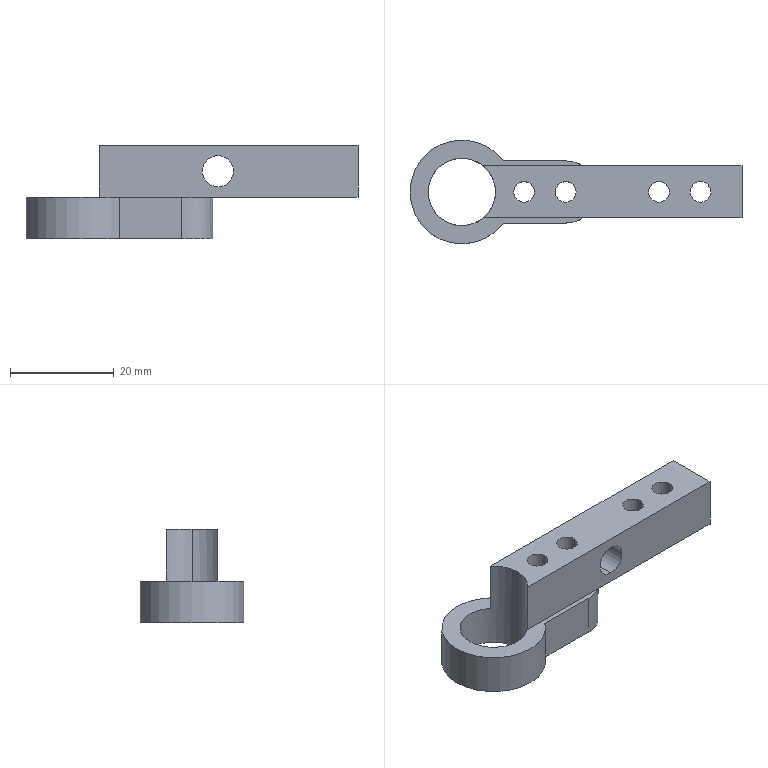Part | SolidWorks | features ICE 6, Extrusion 1 | 1 solid | 24 faces | box 64 x 20 x 18 mm | volume 6760 mm3 | cylinder 15 | plane 9 | commonest cylinder face diameters 4 x8 6 x2 12 x2 13 x2 20 x1
STEP:
#1=CARTESIAN_POINT('',(2.5,5.,10.));
#2=VERTEX_POINT('',#1);
#3=CARTESIAN_POINT('',(0.1533,0.,10.));
#4=VERTEX_POINT('',#3);
#5=CARTESIAN_POINT('',(-4.,5.,10.));
#6=DIRECTION('',(0.,0.,-1.));
#7=DIRECTION('',(-1.,0.,0.));
#8=AXIS2_PLACEMENT_3D('',#5,#6,#7);
#9=CIRCLE('',#8,6.5);
#10=EDGE_CURVE('',#2,#4,#9,.T.);
#11=ORIENTED_EDGE('',*,*,#10,.F.);
#12=CARTESIAN_POINT('',(2.5,5.,-8.));
#13=VERTEX_POINT('',#12);
#14=CARTESIAN_POINT('',(2.5,5.,10.));
#15=DIRECTION('',(0.,0.,-1.));
#16=VECTOR('',#15,1000.);
#17=LINE('',#14,#16);
#18=EDGE_CURVE('',#2,#13,#17,.T.);
#19=ORIENTED_EDGE('',*,*,#18,.T.);
#20=CARTESIAN_POINT('',(-10.5,5.,-8.));
#21=VERTEX_POINT('',#20);
#22=CARTESIAN_POINT('',(-4.,5.,-8.));
#23=DIRECTION('',(0.,0.,1.));
#24=DIRECTION('',(1.,0.,0.));
#25=AXIS2_PLACEMENT_3D('',#22,#23,#24);
#26=CIRCLE('',#25,6.5);
#27=EDGE_CURVE('',#21,#13,#26,.T.);
#28=ORIENTED_EDGE('',*,*,#27,.F.);
#29=CARTESIAN_POINT('',(-10.5,5.,0.));
#30=VERTEX_POINT('',#29);
#31=CARTESIAN_POINT('',(-10.5,5.,10.));
#32=DIRECTION('',(0.,0.,-1.));
#33=VECTOR('',#32,1000.);
#34=LINE('',#31,#33);
#35=EDGE_CURVE('',#30,#21,#34,.T.);
#36=ORIENTED_EDGE('',*,*,#35,.F.);
#37=CARTESIAN_POINT('',(0.1533,0.,0.));
#38=VERTEX_POINT('',#37);
#39=CARTESIAN_POINT('',(-4.,5.,0.));
#40=DIRECTION('',(0.,0.,-1.));
#41=DIRECTION('',(-1.,0.,0.));
#42=AXIS2_PLACEMENT_3D('',#39,#40,#41);
#43=CIRCLE('',#42,6.5);
#44=EDGE_CURVE('',#38,#30,#43,.T.);
#45=ORIENTED_EDGE('',*,*,#44,.F.);
#46=CARTESIAN_POINT('',(0.1533,0.,10.));
#47=DIRECTION('',(0.,0.,-1.));
#48=VECTOR('',#47,1000.);
#49=LINE('',#46,#48);
#50=EDGE_CURVE('',#4,#38,#49,.T.);
#51=ORIENTED_EDGE('',*,*,#50,.F.);
#52=EDGE_LOOP('',(#11,#19,#28,#36,#45,#51));
#53=FACE_OUTER_BOUND('',#52,.T.);
#54=CARTESIAN_POINT('',(-4.,5.,10.));
#55=DIRECTION('',(0.,0.,-1.));
#56=DIRECTION('',(-1.,0.,0.));
#57=AXIS2_PLACEMENT_3D('',#54,#55,#56);
#58=CYLINDRICAL_SURFACE('',#57,6.5);
#59=ADVANCED_FACE('',(#53),#58,.F.);
#60=CARTESIAN_POINT('',(16.,-1.,-8.));
#61=VERTEX_POINT('',#60);
#62=CARTESIAN_POINT('',(22.,5.,-8.));
#63=VERTEX_POINT('',#62);
#64=CARTESIAN_POINT('',(16.,5.,-8.));
#65=DIRECTION('',(0.,0.,1.));
#66=DIRECTION('',(1.,0.,0.));
#67=AXIS2_PLACEMENT_3D('',#64,#65,#66);
#68=CIRCLE('',#67,6.);
#69=EDGE_CURVE('',#61,#63,#68,.T.);
#70=ORIENTED_EDGE('',*,*,#69,.T.);
#71=CARTESIAN_POINT('',(22.,5.,0.));
#72=VERTEX_POINT('',#71);
#73=CARTESIAN_POINT('',(22.,5.,-30.));
#74=DIRECTION('',(0.,0.,1.));
#75=VECTOR('',#74,1000.);
#76=LINE('',#73,#75);
#77=EDGE_CURVE('',#63,#72,#76,.T.);
#78=ORIENTED_EDGE('',*,*,#77,.T.);
#79=CARTESIAN_POINT('',(19.317,0.,0.));
#80=VERTEX_POINT('',#79);
#81=CARTESIAN_POINT('',(16.,5.,0.));
#82=DIRECTION('',(0.,0.,-1.));
#83=DIRECTION('',(-1.,0.,0.));
#84=AXIS2_PLACEMENT_3D('',#81,#82,#83);
#85=CIRCLE('',#84,6.);
#86=EDGE_CURVE('',#72,#80,#85,.T.);
#87=ORIENTED_EDGE('',*,*,#86,.T.);
#88=CARTESIAN_POINT('',(16.,-1.,0.));
#89=VERTEX_POINT('',#88);
#90=CARTESIAN_POINT('',(16.,5.,0.));
#91=DIRECTION('',(0.,0.,-1.));
#92=DIRECTION('',(-1.,0.,0.));
#93=AXIS2_PLACEMENT_3D('',#90,#91,#92);
#94=CIRCLE('',#93,6.);
#95=EDGE_CURVE('',#80,#89,#94,.T.);
#96=ORIENTED_EDGE('',*,*,#95,.T.);
#97=CARTESIAN_POINT('',(16.,-1.,-30.));
#98=DIRECTION('',(0.,0.,1.));
#99=VECTOR('',#98,1000.);
#100=LINE('',#97,#99);
#101=EDGE_CURVE('',#61,#89,#100,.T.);
#102=ORIENTED_EDGE('',*,*,#101,.F.);
#103=EDGE_LOOP('',(#70,#78,#87,#96,#102));
#104=FACE_OUTER_BOUND('',#103,.T.);
#105=CARTESIAN_POINT('',(16.,5.,-30.));
#106=DIRECTION('',(0.,0.,1.));
#107=DIRECTION('',(1.,0.,0.));
#108=AXIS2_PLACEMENT_3D('',#105,#106,#107);
#109=CYLINDRICAL_SURFACE('',#108,6.);
#110=ADVANCED_FACE('',(#104),#109,.T.);
#111=CARTESIAN_POINT('',(6.,5.,-8.));
#112=VERTEX_POINT('',#111);
#113=CARTESIAN_POINT('',(10.,5.,-8.));
#114=VERTEX_POINT('',#113);
#115=CARTESIAN_POINT('',(8.,5.,-8.));
#116=DIRECTION('',(0.,0.,1.));
#117=DIRECTION('',(1.,0.,0.));
#118=AXIS2_PLACEMENT_3D('',#115,#116,#117);
#119=CIRCLE('',#118,2.);
#120=EDGE_CURVE('',#112,#114,#119,.T.);
#121=ORIENTED_EDGE('',*,*,#120,.F.);
#122=CARTESIAN_POINT('',(6.,5.,10.));
#123=VERTEX_POINT('',#122);
#124=CARTESIAN_POINT('',(6.,5.,0.));
#125=DIRECTION('',(0.,0.,1.));
#126=VECTOR('',#125,1000.);
#127=LINE('',#124,#126);
#128=EDGE_CURVE('',#112,#123,#127,.T.);
#129=ORIENTED_EDGE('',*,*,#128,.T.);
#130=CARTESIAN_POINT('',(10.,5.,10.));
#131=VERTEX_POINT('',#130);
#132=CARTESIAN_POINT('',(8.,5.,10.));
#133=DIRECTION('',(0.,0.,1.));
#134=DIRECTION('',(1.,0.,0.));
#135=AXIS2_PLACEMENT_3D('',#132,#133,#134);
#136=CIRCLE('',#135,2.);
#137=EDGE_CURVE('',#123,#131,#136,.T.);
#138=ORIENTED_EDGE('',*,*,#137,.T.);
#139=CARTESIAN_POINT('',(10.,5.,0.));
#140=DIRECTION('',(0.,0.,1.));
#141=VECTOR('',#140,1000.);
#142=LINE('',#139,#141);
#143=EDGE_CURVE('',#114,#131,#142,.T.);
#144=ORIENTED_EDGE('',*,*,#143,.F.);
#145=EDGE_LOOP('',(#121,#129,#138,#144));
#146=FACE_OUTER_BOUND('',#145,.T.);
#147=CARTESIAN_POINT('',(8.,5.,0.));
#148=DIRECTION('',(0.,0.,1.));
#149=DIRECTION('',(1.,0.,0.));
#150=AXIS2_PLACEMENT_3D('',#147,#148,#149);
#151=CYLINDRICAL_SURFACE('',#150,2.);
#152=ADVANCED_FACE('',(#146),#151,.F.);
#153=CARTESIAN_POINT('',(32.,5.,0.));
#154=VERTEX_POINT('',#153);
#155=CARTESIAN_POINT('',(36.,5.,0.));
#156=VERTEX_POINT('',#155);
#157=CARTESIAN_POINT('',(34.,5.,0.));
#158=DIRECTION('',(0.,0.,1.));
#159=DIRECTION('',(-1.,0.,0.));
#160=AXIS2_PLACEMENT_3D('',#157,#158,#159);
#161=CIRCLE('',#160,2.);
#162=EDGE_CURVE('',#154,#156,#161,.T.);
#163=ORIENTED_EDGE('',*,*,#162,.F.);
#164=CARTESIAN_POINT('',(32.,5.,10.));
#165=VERTEX_POINT('',#164);
#166=CARTESIAN_POINT('',(32.,5.,0.));
#167=DIRECTION('',(0.,0.,1.));
#168=VECTOR('',#167,1000.);
#169=LINE('',#166,#168);
#170=EDGE_CURVE('',#154,#165,#169,.T.);
#171=ORIENTED_EDGE('',*,*,#170,.T.);
#172=CARTESIAN_POINT('',(36.,5.,10.));
#173=VERTEX_POINT('',#172);
#174=CARTESIAN_POINT('',(34.,5.,10.));
#175=DIRECTION('',(0.,0.,1.));
#176=DIRECTION('',(-1.,0.,0.));
#177=AXIS2_PLACEMENT_3D('',#174,#175,#176);
#178=CIRCLE('',#177,2.);
#179=EDGE_CURVE('',#165,#173,#178,.T.);
#180=ORIENTED_EDGE('',*,*,#179,.T.);
#181=CARTESIAN_POINT('',(36.,5.,0.));
#182=DIRECTION('',(0.,0.,1.));
#183=VECTOR('',#182,1000.);
#184=LINE('',#181,#183);
#185=EDGE_CURVE('',#156,#173,#184,.T.);
#186=ORIENTED_EDGE('',*,*,#185,.F.);
#187=EDGE_LOOP('',(#163,#171,#180,#186));
#188=FACE_OUTER_BOUND('',#187,.T.);
#189=CARTESIAN_POINT('',(34.,5.,0.));
#190=DIRECTION('',(0.,0.,1.));
#191=DIRECTION('',(1.,0.,0.));
#192=AXIS2_PLACEMENT_3D('',#189,#190,#191);
#193=CYLINDRICAL_SURFACE('',#192,2.);
#194=ADVANCED_FACE('',(#188),#193,.F.);
#195=CARTESIAN_POINT('',(40.,5.,0.));
#196=VERTEX_POINT('',#195);
#197=CARTESIAN_POINT('',(44.,5.,0.));
#198=VERTEX_POINT('',#197);
#199=CARTESIAN_POINT('',(42.,5.,0.));
#200=DIRECTION('',(0.,0.,1.));
#201=DIRECTION('',(-1.,0.,0.));
#202=AXIS2_PLACEMENT_3D('',#199,#200,#201);
#203=CIRCLE('',#202,2.);
#204=EDGE_CURVE('',#196,#198,#203,.T.);
#205=ORIENTED_EDGE('',*,*,#204,.F.);
#206=CARTESIAN_POINT('',(40.,5.,10.));
#207=VERTEX_POINT('',#206);
#208=CARTESIAN_POINT('',(40.,5.,0.));
#209=DIRECTION('',(0.,0.,1.));
#210=VECTOR('',#209,1000.);
#211=LINE('',#208,#210);
#212=EDGE_CURVE('',#196,#207,#211,.T.);
#213=ORIENTED_EDGE('',*,*,#212,.T.);
#214=CARTESIAN_POINT('',(44.,5.,10.));
#215=VERTEX_POINT('',#214);
#216=CARTESIAN_POINT('',(42.,5.,10.));
#217=DIRECTION('',(0.,0.,1.));
#218=DIRECTION('',(-1.,0.,0.));
#219=AXIS2_PLACEMENT_3D('',#216,#217,#218);
#220=CIRCLE('',#219,2.);
#221=EDGE_CURVE('',#207,#215,#220,.T.);
#222=ORIENTED_EDGE('',*,*,#221,.T.);
#223=CARTESIAN_POINT('',(44.,5.,0.));
#224=DIRECTION('',(0.,0.,1.));
#225=VECTOR('',#224,1000.);
#226=LINE('',#223,#225);
#227=EDGE_CURVE('',#198,#215,#226,.T.);
#228=ORIENTED_EDGE('',*,*,#227,.F.);
#229=EDGE_LOOP('',(#205,#213,#222,#228));
#230=FACE_OUTER_BOUND('',#229,.T.);
#231=CARTESIAN_POINT('',(42.,5.,0.));
#232=DIRECTION('',(0.,0.,1.));
#233=DIRECTION('',(1.,0.,0.));
#234=AXIS2_PLACEMENT_3D('',#231,#232,#233);
#235=CYLINDRICAL_SURFACE('',#234,2.);
#236=ADVANCED_FACE('',(#230),#235,.F.);
#237=CARTESIAN_POINT('',(14.,5.,-8.));
#238=VERTEX_POINT('',#237);
#239=CARTESIAN_POINT('',(18.,5.,-8.));
#240=VERTEX_POINT('',#239);
#241=CARTESIAN_POINT('',(16.,5.,-8.));
#242=DIRECTION('',(0.,0.,1.));
#243=DIRECTION('',(1.,0.,0.));
#244=AXIS2_PLACEMENT_3D('',#241,#242,#243);
#245=CIRCLE('',#244,2.);
#246=EDGE_CURVE('',#238,#240,#245,.T.);
#247=ORIENTED_EDGE('',*,*,#246,.F.);
#248=CARTESIAN_POINT('',(14.,5.,10.));
#249=VERTEX_POINT('',#248);
#250=CARTESIAN_POINT('',(14.,5.,0.));
#251=DIRECTION('',(0.,0.,1.));
#252=VECTOR('',#251,1000.);
#253=LINE('',#250,#252);
#254=EDGE_CURVE('',#238,#249,#253,.T.);
#255=ORIENTED_EDGE('',*,*,#254,.T.);
#256=CARTESIAN_POINT('',(18.,5.,10.));
#257=VERTEX_POINT('',#256);
#258=CARTESIAN_POINT('',(16.,5.,10.));
#259=DIRECTION('',(0.,0.,1.));
#260=DIRECTION('',(1.,0.,0.));
#261=AXIS2_PLACEMENT_3D('',#258,#259,#260);
#262=CIRCLE('',#261,2.);
#263=EDGE_CURVE('',#249,#257,#262,.T.);
#264=ORIENTED_EDGE('',*,*,#263,.T.);
#265=CARTESIAN_POINT('',(18.,5.,0.));
#266=DIRECTION('',(0.,0.,1.));
#267=VECTOR('',#266,1000.);
#268=LINE('',#265,#267);
#269=EDGE_CURVE('',#240,#257,#268,.T.);
#270=ORIENTED_EDGE('',*,*,#269,.F.);
#271=EDGE_LOOP('',(#247,#255,#264,#270));
#272=FACE_OUTER_BOUND('',#271,.T.);
#273=CARTESIAN_POINT('',(16.,5.,0.));
#274=DIRECTION('',(0.,0.,1.));
#275=DIRECTION('',(1.,0.,0.));
#276=AXIS2_PLACEMENT_3D('',#273,#274,#275);
#277=CYLINDRICAL_SURFACE('',#276,2.);
#278=ADVANCED_FACE('',(#272),#277,.F.);
#279=CARTESIAN_POINT('',(23.,0.,2.));
#280=VERTEX_POINT('',#279);
#281=CARTESIAN_POINT('',(23.,0.,8.));
#282=VERTEX_POINT('',#281);
#283=CARTESIAN_POINT('',(23.,0.,5.));
#284=DIRECTION('',(0.,1.,0.));
#285=DIRECTION('',(0.,0.,1.));
#286=AXIS2_PLACEMENT_3D('',#283,#284,#285);
#287=CIRCLE('',#286,3.);
#288=EDGE_CURVE('',#280,#282,#287,.T.);
#289=ORIENTED_EDGE('',*,*,#288,.F.);
#290=CARTESIAN_POINT('',(23.,10.,2.));
#291=VERTEX_POINT('',#290);
#292=CARTESIAN_POINT('',(23.,0.,2.));
#293=DIRECTION('',(0.,1.,0.));
#294=VECTOR('',#293,1000.);
#295=LINE('',#292,#294);
#296=EDGE_CURVE('',#280,#291,#295,.T.);
#297=ORIENTED_EDGE('',*,*,#296,.T.);
#298=CARTESIAN_POINT('',(23.,10.,8.));
#299=VERTEX_POINT('',#298);
#300=CARTESIAN_POINT('',(23.,10.,5.));
#301=DIRECTION('',(0.,1.,0.));
#302=DIRECTION('',(0.,0.,1.));
#303=AXIS2_PLACEMENT_3D('',#300,#301,#302);
#304=CIRCLE('',#303,3.);
#305=EDGE_CURVE('',#291,#299,#304,.T.);
#306=ORIENTED_EDGE('',*,*,#305,.T.);
#307=CARTESIAN_POINT('',(23.,0.,8.));
#308=DIRECTION('',(0.,1.,0.));
#309=VECTOR('',#308,1000.);
#310=LINE('',#307,#309);
#311=EDGE_CURVE('',#282,#299,#310,.T.);
#312=ORIENTED_EDGE('',*,*,#311,.F.);
#313=EDGE_LOOP('',(#289,#297,#306,#312));
#314=FACE_OUTER_BOUND('',#313,.T.);
#315=CARTESIAN_POINT('',(23.,0.,5.));
#316=DIRECTION('',(0.,1.,0.));
#317=DIRECTION('',(0.,0.,1.));
#318=AXIS2_PLACEMENT_3D('',#315,#316,#317);
#319=CYLINDRICAL_SURFACE('',#318,3.);
#320=ADVANCED_FACE('',(#314),#319,.F.);
#321=CARTESIAN_POINT('',(8.,5.,10.));
#322=DIRECTION('',(0.,0.,1.));
#323=DIRECTION('',(1.,0.,0.));
#324=AXIS2_PLACEMENT_3D('',#321,#322,#323);
#325=CIRCLE('',#324,2.);
#326=EDGE_CURVE('',#131,#123,#325,.T.);
#327=ORIENTED_EDGE('',*,*,#326,.F.);
#328=ORIENTED_EDGE('',*,*,#137,.F.);
#329=EDGE_LOOP('',(#327,#328));
#330=FACE_BOUND('',#329,.T.);
#331=CARTESIAN_POINT('',(34.,5.,10.));
#332=DIRECTION('',(0.,0.,1.));
#333=DIRECTION('',(-1.,0.,0.));
#334=AXIS2_PLACEMENT_3D('',#331,#332,#333);
#335=CIRCLE('',#334,2.);
#336=EDGE_CURVE('',#173,#165,#335,.T.);
#337=ORIENTED_EDGE('',*,*,#336,.F.);
#338=ORIENTED_EDGE('',*,*,#179,.F.);
#339=EDGE_LOOP('',(#337,#338));
#340=FACE_BOUND('',#339,.T.);
#341=CARTESIAN_POINT('',(42.,5.,10.));
#342=DIRECTION('',(0.,0.,1.));
#343=DIRECTION('',(-1.,0.,0.));
#344=AXIS2_PLACEMENT_3D('',#341,#342,#343);
#345=CIRCLE('',#344,2.);
#346=EDGE_CURVE('',#215,#207,#345,.T.);
#347=ORIENTED_EDGE('',*,*,#346,.F.);
#348=ORIENTED_EDGE('',*,*,#221,.F.);
#349=EDGE_LOOP('',(#347,#348));
#350=FACE_BOUND('',#349,.T.);
#351=CARTESIAN_POINT('',(16.,5.,10.));
#352=DIRECTION('',(0.,0.,1.));
#353=DIRECTION('',(1.,0.,0.));
#354=AXIS2_PLACEMENT_3D('',#351,#352,#353);
#355=CIRCLE('',#354,2.);
#356=EDGE_CURVE('',#257,#249,#355,.T.);
#357=ORIENTED_EDGE('',*,*,#356,.F.);
#358=ORIENTED_EDGE('',*,*,#263,.F.);
#359=EDGE_LOOP('',(#357,#358));
#360=FACE_BOUND('',#359,.T.);
#361=CARTESIAN_POINT('',(0.1533,10.,10.));
#362=VERTEX_POINT('',#361);
#363=CARTESIAN_POINT('',(50.,10.,10.));
#364=VERTEX_POINT('',#363);
#365=CARTESIAN_POINT('',(0.,10.,10.));
#366=DIRECTION('',(1.,0.,0.));
#367=VECTOR('',#366,1000.);
#368=LINE('',#365,#367);
#369=EDGE_CURVE('',#362,#364,#368,.T.);
#370=ORIENTED_EDGE('',*,*,#369,.F.);
#371=CARTESIAN_POINT('',(-4.,5.,10.));
#372=DIRECTION('',(0.,0.,-1.));
#373=DIRECTION('',(-1.,0.,0.));
#374=AXIS2_PLACEMENT_3D('',#371,#372,#373);
#375=CIRCLE('',#374,6.5);
#376=EDGE_CURVE('',#362,#2,#375,.T.);
#377=ORIENTED_EDGE('',*,*,#376,.T.);
#378=ORIENTED_EDGE('',*,*,#10,.T.);
#379=CARTESIAN_POINT('',(50.,0.,10.));
#380=VERTEX_POINT('',#379);
#381=CARTESIAN_POINT('',(0.,0.,10.));
#382=DIRECTION('',(1.,0.,0.));
#383=VECTOR('',#382,1000.);
#384=LINE('',#381,#383);
#385=EDGE_CURVE('',#4,#380,#384,.T.);
#386=ORIENTED_EDGE('',*,*,#385,.T.);
#387=CARTESIAN_POINT('',(50.,10.,10.));
#388=DIRECTION('',(0.,-1.,0.));
#389=VECTOR('',#388,1000.);
#390=LINE('',#387,#389);
#391=EDGE_CURVE('',#364,#380,#390,.T.);
#392=ORIENTED_EDGE('',*,*,#391,.F.);
#393=EDGE_LOOP('',(#370,#377,#378,#386,#392));
#394=FACE_OUTER_BOUND('',#393,.T.);
#395=CARTESIAN_POINT('',(0.,10.,10.));
#396=DIRECTION('',(0.,0.,-1.));
#397=DIRECTION('',(-1.,0.,0.));
#398=AXIS2_PLACEMENT_3D('',#395,#396,#397);
#399=PLANE('',#398);
#400=ADVANCED_FACE('',(#330,#340,#350,#360,#394),#399,.F.);
#401=CARTESIAN_POINT('',(50.,0.,0.));
#402=VERTEX_POINT('',#401);
#403=CARTESIAN_POINT('',(50.,0.,0.));
#404=DIRECTION('',(0.,0.,-1.));
#405=VECTOR('',#404,1000.);
#406=LINE('',#403,#405);
#407=EDGE_CURVE('',#380,#402,#406,.T.);
#408=ORIENTED_EDGE('',*,*,#407,.T.);
#409=CARTESIAN_POINT('',(50.,10.,0.));
#410=VERTEX_POINT('',#409);
#411=CARTESIAN_POINT('',(50.,10.,0.));
#412=DIRECTION('',(0.,-1.,0.));
#413=VECTOR('',#412,1000.);
#414=LINE('',#411,#413);
#415=EDGE_CURVE('',#410,#402,#414,.T.);
#416=ORIENTED_EDGE('',*,*,#415,.F.);
#417=CARTESIAN_POINT('',(50.,10.,0.));
#418=DIRECTION('',(0.,0.,-1.));
#419=VECTOR('',#418,1000.);
#420=LINE('',#417,#419);
#421=EDGE_CURVE('',#364,#410,#420,.T.);
#422=ORIENTED_EDGE('',*,*,#421,.F.);
#423=ORIENTED_EDGE('',*,*,#391,.T.);
#424=EDGE_LOOP('',(#408,#416,#422,#423));
#425=FACE_OUTER_BOUND('',#424,.T.);
#426=CARTESIAN_POINT('',(50.,10.,0.));
#427=DIRECTION('',(-1.,0.,0.));
#428=DIRECTION('',(0.,0.,1.));
#429=AXIS2_PLACEMENT_3D('',#426,#427,#428);
#430=PLANE('',#429);
#431=ADVANCED_FACE('',(#425),#430,.F.);
#432=CARTESIAN_POINT('',(19.317,10.,0.));
#433=VERTEX_POINT('',#432);
#434=CARTESIAN_POINT('',(16.,5.,0.));
#435=DIRECTION('',(0.,0.,-1.));
#436=DIRECTION('',(-1.,0.,0.));
#437=AXIS2_PLACEMENT_3D('',#434,#435,#436);
#438=CIRCLE('',#437,6.);
#439=EDGE_CURVE('',#433,#72,#438,.T.);
#440=ORIENTED_EDGE('',*,*,#439,.F.);
#441=CARTESIAN_POINT('',(0.,10.,0.));
#442=DIRECTION('',(-1.,0.,0.));
#443=VECTOR('',#442,1000.);
#444=LINE('',#441,#443);
#445=EDGE_CURVE('',#410,#433,#444,.T.);
#446=ORIENTED_EDGE('',*,*,#445,.F.);
#447=ORIENTED_EDGE('',*,*,#415,.T.);
#448=CARTESIAN_POINT('',(0.,0.,0.));
#449=DIRECTION('',(-1.,0.,0.));
#450=VECTOR('',#449,1000.);
#451=LINE('',#448,#450);
#452=EDGE_CURVE('',#402,#80,#451,.T.);
#453=ORIENTED_EDGE('',*,*,#452,.T.);
#454=ORIENTED_EDGE('',*,*,#86,.F.);
#455=EDGE_LOOP('',(#440,#446,#447,#453,#454));
#456=FACE_OUTER_BOUND('',#455,.T.);
#457=CARTESIAN_POINT('',(34.,5.,0.));
#458=DIRECTION('',(0.,0.,1.));
#459=DIRECTION('',(-1.,0.,0.));
#460=AXIS2_PLACEMENT_3D('',#457,#458,#459);
#461=CIRCLE('',#460,2.);
#462=EDGE_CURVE('',#156,#154,#461,.T.);
#463=ORIENTED_EDGE('',*,*,#462,.T.);
#464=ORIENTED_EDGE('',*,*,#162,.T.);
#465=EDGE_LOOP('',(#463,#464));
#466=FACE_BOUND('',#465,.T.);
#467=CARTESIAN_POINT('',(42.,5.,0.));
#468=DIRECTION('',(0.,0.,1.));
#469=DIRECTION('',(-1.,0.,0.));
#470=AXIS2_PLACEMENT_3D('',#467,#468,#469);
#471=CIRCLE('',#470,2.);
#472=EDGE_CURVE('',#198,#196,#471,.T.);
#473=ORIENTED_EDGE('',*,*,#472,.T.);
#474=ORIENTED_EDGE('',*,*,#204,.T.);
#475=EDGE_LOOP('',(#473,#474));
#476=FACE_BOUND('',#475,.T.);
#477=CARTESIAN_POINT('',(0.,10.,0.));
#478=DIRECTION('',(0.,0.,1.));
#479=DIRECTION('',(1.,0.,0.));
#480=AXIS2_PLACEMENT_3D('',#477,#478,#479);
#481=PLANE('',#480);
#482=ADVANCED_FACE('',(#456,#466,#476),#481,.F.);
#483=CARTESIAN_POINT('',(0.1533,10.,0.));
#484=VERTEX_POINT('',#483);
#485=CARTESIAN_POINT('',(0.1533,10.,10.));
#486=DIRECTION('',(0.,0.,-1.));
#487=VECTOR('',#486,1000.);
#488=LINE('',#485,#487);
#489=EDGE_CURVE('',#362,#484,#488,.T.);
#490=ORIENTED_EDGE('',*,*,#489,.F.);
#491=ORIENTED_EDGE('',*,*,#369,.T.);
#492=ORIENTED_EDGE('',*,*,#421,.T.);
#493=ORIENTED_EDGE('',*,*,#445,.T.);
#494=CARTESIAN_POINT('',(0.,10.,0.));
#495=DIRECTION('',(-1.,0.,0.));
#496=VECTOR('',#495,1000.);
#497=LINE('',#494,#496);
#498=EDGE_CURVE('',#433,#484,#497,.T.);
#499=ORIENTED_EDGE('',*,*,#498,.T.);
#500=EDGE_LOOP('',(#490,#491,#492,#493,#499));
#501=FACE_OUTER_BOUND('',#500,.T.);
#502=CARTESIAN_POINT('',(23.,10.,5.));
#503=DIRECTION('',(0.,1.,0.));
#504=DIRECTION('',(0.,0.,1.));
#505=AXIS2_PLACEMENT_3D('',#502,#503,#504);
#506=CIRCLE('',#505,3.);
#507=EDGE_CURVE('',#299,#291,#506,.T.);
#508=ORIENTED_EDGE('',*,*,#507,.F.);
#509=ORIENTED_EDGE('',*,*,#305,.F.);
#510=EDGE_LOOP('',(#508,#509));
#511=FACE_BOUND('',#510,.T.);
#512=CARTESIAN_POINT('',(0.,10.,0.));
#513=DIRECTION('',(0.,1.,0.));
#514=DIRECTION('',(0.,0.,1.));
#515=AXIS2_PLACEMENT_3D('',#512,#513,#514);
#516=PLANE('',#515);
#517=ADVANCED_FACE('',(#501,#511),#516,.T.);
#518=CARTESIAN_POINT('',(23.,0.,5.));
#519=DIRECTION('',(0.,1.,0.));
#520=DIRECTION('',(0.,0.,1.));
#521=AXIS2_PLACEMENT_3D('',#518,#519,#520);
#522=CIRCLE('',#521,3.);
#523=EDGE_CURVE('',#282,#280,#522,.T.);
#524=ORIENTED_EDGE('',*,*,#523,.T.);
#525=ORIENTED_EDGE('',*,*,#288,.T.);
#526=EDGE_LOOP('',(#524,#525));
#527=FACE_BOUND('',#526,.T.);
#528=ORIENTED_EDGE('',*,*,#385,.F.);
#529=ORIENTED_EDGE('',*,*,#50,.T.);
#530=CARTESIAN_POINT('',(0.,0.,0.));
#531=DIRECTION('',(-1.,0.,0.));
#532=VECTOR('',#531,1000.);
#533=LINE('',#530,#532);
#534=EDGE_CURVE('',#80,#38,#533,.T.);
#535=ORIENTED_EDGE('',*,*,#534,.F.);
#536=ORIENTED_EDGE('',*,*,#452,.F.);
#537=ORIENTED_EDGE('',*,*,#407,.F.);
#538=EDGE_LOOP('',(#528,#529,#535,#536,#537));
#539=FACE_OUTER_BOUND('',#538,.T.);
#540=CARTESIAN_POINT('',(0.,0.,0.));
#541=DIRECTION('',(0.,1.,0.));
#542=DIRECTION('',(0.,0.,1.));
#543=AXIS2_PLACEMENT_3D('',#540,#541,#542);
#544=PLANE('',#543);
#545=ADVANCED_FACE('',(#527,#539),#544,.F.);
#546=ORIENTED_EDGE('',*,*,#296,.F.);
#547=ORIENTED_EDGE('',*,*,#523,.F.);
#548=ORIENTED_EDGE('',*,*,#311,.T.);
#549=ORIENTED_EDGE('',*,*,#507,.T.);
#550=EDGE_LOOP('',(#546,#547,#548,#549));
#551=FACE_OUTER_BOUND('',#550,.T.);
#552=CARTESIAN_POINT('',(23.,0.,5.));
#553=DIRECTION('',(0.,1.,0.));
#554=DIRECTION('',(0.,0.,1.));
#555=AXIS2_PLACEMENT_3D('',#552,#553,#554);
#556=CYLINDRICAL_SURFACE('',#555,3.);
#557=ADVANCED_FACE('',(#551),#556,.F.);
#558=ORIENTED_EDGE('',*,*,#254,.F.);
#559=CARTESIAN_POINT('',(16.,5.,-8.));
#560=DIRECTION('',(0.,0.,1.));
#561=DIRECTION('',(1.,0.,0.));
#562=AXIS2_PLACEMENT_3D('',#559,#560,#561);
#563=CIRCLE('',#562,2.);
#564=EDGE_CURVE('',#240,#238,#563,.T.);
#565=ORIENTED_EDGE('',*,*,#564,.F.);
#566=ORIENTED_EDGE('',*,*,#269,.T.);
#567=ORIENTED_EDGE('',*,*,#356,.T.);
#568=EDGE_LOOP('',(#558,#565,#566,#567));
#569=FACE_OUTER_BOUND('',#568,.T.);
#570=CARTESIAN_POINT('',(16.,5.,0.));
#571=DIRECTION('',(0.,0.,1.));
#572=DIRECTION('',(1.,0.,0.));
#573=AXIS2_PLACEMENT_3D('',#570,#571,#572);
#574=CYLINDRICAL_SURFACE('',#573,2.);
#575=ADVANCED_FACE('',(#569),#574,.F.);
#576=ORIENTED_EDGE('',*,*,#212,.F.);
#577=ORIENTED_EDGE('',*,*,#472,.F.);
#578=ORIENTED_EDGE('',*,*,#227,.T.);
#579=ORIENTED_EDGE('',*,*,#346,.T.);
#580=EDGE_LOOP('',(#576,#577,#578,#579));
#581=FACE_OUTER_BOUND('',#580,.T.);
#582=CARTESIAN_POINT('',(42.,5.,0.));
#583=DIRECTION('',(0.,0.,1.));
#584=DIRECTION('',(1.,0.,0.));
#585=AXIS2_PLACEMENT_3D('',#582,#583,#584);
#586=CYLINDRICAL_SURFACE('',#585,2.);
#587=ADVANCED_FACE('',(#581),#586,.F.);
#588=ORIENTED_EDGE('',*,*,#170,.F.);
#589=ORIENTED_EDGE('',*,*,#462,.F.);
#590=ORIENTED_EDGE('',*,*,#185,.T.);
#591=ORIENTED_EDGE('',*,*,#336,.T.);
#592=EDGE_LOOP('',(#588,#589,#590,#591));
#593=FACE_OUTER_BOUND('',#592,.T.);
#594=CARTESIAN_POINT('',(34.,5.,0.));
#595=DIRECTION('',(0.,0.,1.));
#596=DIRECTION('',(1.,0.,0.));
#597=AXIS2_PLACEMENT_3D('',#594,#595,#596);
#598=CYLINDRICAL_SURFACE('',#597,2.);
#599=ADVANCED_FACE('',(#593),#598,.F.);
#600=ORIENTED_EDGE('',*,*,#128,.F.);
#601=CARTESIAN_POINT('',(8.,5.,-8.));
#602=DIRECTION('',(0.,0.,1.));
#603=DIRECTION('',(1.,0.,0.));
#604=AXIS2_PLACEMENT_3D('',#601,#602,#603);
#605=CIRCLE('',#604,2.);
#606=EDGE_CURVE('',#114,#112,#605,.T.);
#607=ORIENTED_EDGE('',*,*,#606,.F.);
#608=ORIENTED_EDGE('',*,*,#143,.T.);
#609=ORIENTED_EDGE('',*,*,#326,.T.);
#610=EDGE_LOOP('',(#600,#607,#608,#609));
#611=FACE_OUTER_BOUND('',#610,.T.);
#612=CARTESIAN_POINT('',(8.,5.,0.));
#613=DIRECTION('',(0.,0.,1.));
#614=DIRECTION('',(1.,0.,0.));
#615=AXIS2_PLACEMENT_3D('',#612,#613,#614);
#616=CYLINDRICAL_SURFACE('',#615,2.);
#617=ADVANCED_FACE('',(#611),#616,.F.);
#618=CARTESIAN_POINT('',(4.,-1.,-8.));
#619=VERTEX_POINT('',#618);
#620=CARTESIAN_POINT('',(4.,-1.,0.));
#621=VERTEX_POINT('',#620);
#622=CARTESIAN_POINT('',(4.,-1.,-30.));
#623=DIRECTION('',(0.,0.,1.));
#624=VECTOR('',#623,1000.);
#625=LINE('',#622,#624);
#626=EDGE_CURVE('',#619,#621,#625,.T.);
#627=ORIENTED_EDGE('',*,*,#626,.F.);
#628=CARTESIAN_POINT('',(16.,-1.,-8.));
#629=DIRECTION('',(1.,0.,0.));
#630=VECTOR('',#629,1000.);
#631=LINE('',#628,#630);
#632=EDGE_CURVE('',#619,#61,#631,.T.);
#633=ORIENTED_EDGE('',*,*,#632,.T.);
#634=ORIENTED_EDGE('',*,*,#101,.T.);
#635=CARTESIAN_POINT('',(16.,-1.,0.));
#636=DIRECTION('',(-1.,0.,0.));
#637=VECTOR('',#636,1000.);
#638=LINE('',#635,#637);
#639=EDGE_CURVE('',#89,#621,#638,.T.);
#640=ORIENTED_EDGE('',*,*,#639,.T.);
#641=EDGE_LOOP('',(#627,#633,#634,#640));
#642=FACE_OUTER_BOUND('',#641,.T.);
#643=CARTESIAN_POINT('',(16.,-1.,-30.));
#644=DIRECTION('',(0.,1.,0.));
#645=DIRECTION('',(-1.,0.,0.));
#646=AXIS2_PLACEMENT_3D('',#643,#644,#645);
#647=PLANE('',#646);
#648=ADVANCED_FACE('',(#642),#647,.F.);
#649=ORIENTED_EDGE('',*,*,#77,.F.);
#650=CARTESIAN_POINT('',(16.,11.,-8.));
#651=VERTEX_POINT('',#650);
#652=CARTESIAN_POINT('',(16.,5.,-8.));
#653=DIRECTION('',(0.,0.,1.));
#654=DIRECTION('',(1.,0.,0.));
#655=AXIS2_PLACEMENT_3D('',#652,#653,#654);
#656=CIRCLE('',#655,6.);
#657=EDGE_CURVE('',#63,#651,#656,.T.);
#658=ORIENTED_EDGE('',*,*,#657,.T.);
#659=CARTESIAN_POINT('',(16.,11.,0.));
#660=VERTEX_POINT('',#659);
#661=CARTESIAN_POINT('',(16.,11.,-30.));
#662=DIRECTION('',(0.,0.,1.));
#663=VECTOR('',#662,1000.);
#664=LINE('',#661,#663);
#665=EDGE_CURVE('',#651,#660,#664,.T.);
#666=ORIENTED_EDGE('',*,*,#665,.T.);
#667=CARTESIAN_POINT('',(16.,5.,0.));
#668=DIRECTION('',(0.,0.,-1.));
#669=DIRECTION('',(-1.,0.,0.));
#670=AXIS2_PLACEMENT_3D('',#667,#668,#669);
#671=CIRCLE('',#670,6.);
#672=EDGE_CURVE('',#660,#433,#671,.T.);
#673=ORIENTED_EDGE('',*,*,#672,.T.);
#674=ORIENTED_EDGE('',*,*,#439,.T.);
#675=EDGE_LOOP('',(#649,#658,#666,#673,#674));
#676=FACE_OUTER_BOUND('',#675,.T.);
#677=CARTESIAN_POINT('',(16.,5.,-30.));
#678=DIRECTION('',(0.,0.,1.));
#679=DIRECTION('',(1.,0.,0.));
#680=AXIS2_PLACEMENT_3D('',#677,#678,#679);
#681=CYLINDRICAL_SURFACE('',#680,6.);
#682=ADVANCED_FACE('',(#676),#681,.T.);
#683=ORIENTED_EDGE('',*,*,#665,.F.);
#684=CARTESIAN_POINT('',(4.,11.,-8.));
#685=VERTEX_POINT('',#684);
#686=CARTESIAN_POINT('',(16.,11.,-8.));
#687=DIRECTION('',(-1.,0.,0.));
#688=VECTOR('',#687,1000.);
#689=LINE('',#686,#688);
#690=EDGE_CURVE('',#651,#685,#689,.T.);
#691=ORIENTED_EDGE('',*,*,#690,.T.);
#692=CARTESIAN_POINT('',(4.,11.,0.));
#693=VERTEX_POINT('',#692);
#694=CARTESIAN_POINT('',(4.,11.,-30.));
#695=DIRECTION('',(0.,0.,1.));
#696=VECTOR('',#695,1000.);
#697=LINE('',#694,#696);
#698=EDGE_CURVE('',#685,#693,#697,.T.);
#699=ORIENTED_EDGE('',*,*,#698,.T.);
#700=CARTESIAN_POINT('',(16.,11.,0.));
#701=DIRECTION('',(1.,0.,0.));
#702=VECTOR('',#701,1000.);
#703=LINE('',#700,#702);
#704=EDGE_CURVE('',#693,#660,#703,.T.);
#705=ORIENTED_EDGE('',*,*,#704,.T.);
#706=EDGE_LOOP('',(#683,#691,#699,#705));
#707=FACE_OUTER_BOUND('',#706,.T.);
#708=CARTESIAN_POINT('',(16.,11.,-30.));
#709=DIRECTION('',(0.,-1.,0.));
#710=DIRECTION('',(0.,0.,-1.));
#711=AXIS2_PLACEMENT_3D('',#708,#709,#710);
#712=PLANE('',#711);
#713=ADVANCED_FACE('',(#707),#712,.F.);
#714=ORIENTED_EDGE('',*,*,#698,.F.);
#715=CARTESIAN_POINT('',(-4.,5.,-8.));
#716=DIRECTION('',(0.,0.,1.));
#717=DIRECTION('',(1.,0.,0.));
#718=AXIS2_PLACEMENT_3D('',#715,#716,#717);
#719=CIRCLE('',#718,10.);
#720=EDGE_CURVE('',#685,#619,#719,.T.);
#721=ORIENTED_EDGE('',*,*,#720,.T.);
#722=ORIENTED_EDGE('',*,*,#626,.T.);
#723=CARTESIAN_POINT('',(-4.,5.,0.));
#724=DIRECTION('',(0.,0.,-1.));
#725=DIRECTION('',(-1.,0.,0.));
#726=AXIS2_PLACEMENT_3D('',#723,#724,#725);
#727=CIRCLE('',#726,10.);
#728=EDGE_CURVE('',#621,#693,#727,.T.);
#729=ORIENTED_EDGE('',*,*,#728,.T.);
#730=EDGE_LOOP('',(#714,#721,#722,#729));
#731=FACE_OUTER_BOUND('',#730,.T.);
#732=CARTESIAN_POINT('',(-4.,5.,-30.));
#733=DIRECTION('',(0.,0.,1.));
#734=DIRECTION('',(1.,0.,0.));
#735=AXIS2_PLACEMENT_3D('',#732,#733,#734);
#736=CYLINDRICAL_SURFACE('',#735,10.);
#737=ADVANCED_FACE('',(#731),#736,.T.);
#738=ORIENTED_EDGE('',*,*,#534,.T.);
#739=ORIENTED_EDGE('',*,*,#44,.T.);
#740=CARTESIAN_POINT('',(-4.,5.,0.));
#741=DIRECTION('',(0.,0.,-1.));
#742=DIRECTION('',(-1.,0.,0.));
#743=AXIS2_PLACEMENT_3D('',#740,#741,#742);
#744=CIRCLE('',#743,6.5);
#745=EDGE_CURVE('',#30,#484,#744,.T.);
#746=ORIENTED_EDGE('',*,*,#745,.T.);
#747=ORIENTED_EDGE('',*,*,#498,.F.);
#748=ORIENTED_EDGE('',*,*,#672,.F.);
#749=ORIENTED_EDGE('',*,*,#704,.F.);
#750=ORIENTED_EDGE('',*,*,#728,.F.);
#751=ORIENTED_EDGE('',*,*,#639,.F.);
#752=ORIENTED_EDGE('',*,*,#95,.F.);
#753=EDGE_LOOP('',(#738,#739,#746,#747,#748,#749,#750,#751,#752));
#754=FACE_OUTER_BOUND('',#753,.T.);
#755=CARTESIAN_POINT('',(-4.,5.,0.));
#756=DIRECTION('',(0.,0.,-1.));
#757=DIRECTION('',(-1.,0.,0.));
#758=AXIS2_PLACEMENT_3D('',#755,#756,#757);
#759=PLANE('',#758);
#760=ADVANCED_FACE('',(#754),#759,.F.);
#761=ORIENTED_EDGE('',*,*,#27,.T.);
#762=CARTESIAN_POINT('',(-4.,5.,-8.));
#763=DIRECTION('',(0.,0.,1.));
#764=DIRECTION('',(1.,0.,0.));
#765=AXIS2_PLACEMENT_3D('',#762,#763,#764);
#766=CIRCLE('',#765,6.5);
#767=EDGE_CURVE('',#13,#21,#766,.T.);
#768=ORIENTED_EDGE('',*,*,#767,.T.);
#769=EDGE_LOOP('',(#761,#768));
#770=FACE_BOUND('',#769,.T.);
#771=ORIENTED_EDGE('',*,*,#606,.T.);
#772=ORIENTED_EDGE('',*,*,#120,.T.);
#773=EDGE_LOOP('',(#771,#772));
#774=FACE_BOUND('',#773,.T.);
#775=ORIENTED_EDGE('',*,*,#564,.T.);
#776=ORIENTED_EDGE('',*,*,#246,.T.);
#777=EDGE_LOOP('',(#775,#776));
#778=FACE_BOUND('',#777,.T.);
#779=ORIENTED_EDGE('',*,*,#720,.F.);
#780=ORIENTED_EDGE('',*,*,#690,.F.);
#781=ORIENTED_EDGE('',*,*,#657,.F.);
#782=ORIENTED_EDGE('',*,*,#69,.F.);
#783=ORIENTED_EDGE('',*,*,#632,.F.);
#784=EDGE_LOOP('',(#779,#780,#781,#782,#783));
#785=FACE_OUTER_BOUND('',#784,.T.);
#786=CARTESIAN_POINT('',(27.691,15.,-8.));
#787=DIRECTION('',(0.,0.,1.));
#788=DIRECTION('',(1.,0.,0.));
#789=AXIS2_PLACEMENT_3D('',#786,#787,#788);
#790=PLANE('',#789);
#791=ADVANCED_FACE('',(#770,#774,#778,#785),#790,.F.);
#792=ORIENTED_EDGE('',*,*,#18,.F.);
#793=ORIENTED_EDGE('',*,*,#376,.F.);
#794=ORIENTED_EDGE('',*,*,#489,.T.);
#795=ORIENTED_EDGE('',*,*,#745,.F.);
#796=ORIENTED_EDGE('',*,*,#35,.T.);
#797=ORIENTED_EDGE('',*,*,#767,.F.);
#798=EDGE_LOOP('',(#792,#793,#794,#795,#796,#797));
#799=FACE_OUTER_BOUND('',#798,.T.);
#800=CARTESIAN_POINT('',(-4.,5.,10.));
#801=DIRECTION('',(0.,0.,-1.));
#802=DIRECTION('',(-1.,0.,0.));
#803=AXIS2_PLACEMENT_3D('',#800,#801,#802);
#804=CYLINDRICAL_SURFACE('',#803,6.5);
#805=ADVANCED_FACE('',(#799),#804,.F.);
#806=CLOSED_SHELL('',(#59,#110,#152,#194,#236,#278,#320,#400,#431,#482,#517,#545,#557,#575,#587,#599,#617,#648,#682,#713,#737,#760,#791,#805));
#807=MANIFOLD_SOLID_BREP('',#806);
#808=CARTESIAN_POINT('',(0.,0.,0.));
#809=DIRECTION('',(0.,0.,1.));
#810=DIRECTION('',(1.,0.,0.));
#811=AXIS2_PLACEMENT_3D('',#808,#809,#810);
#812=(LENGTH_UNIT()NAMED_UNIT(*)SI_UNIT(.MILLI.,.METRE.));
#813=UNCERTAINTY_MEASURE_WITH_UNIT(LENGTH_MEASURE(0.00001),#812,'','');
#814=(NAMED_UNIT(*)PLANE_ANGLE_UNIT()SI_UNIT($,.RADIAN.));
#815=(NAMED_UNIT(*)SI_UNIT($,.STERADIAN.)SOLID_ANGLE_UNIT());
#816=(GEOMETRIC_REPRESENTATION_CONTEXT(3)GLOBAL_UNCERTAINTY_ASSIGNED_CONTEXT((#813))GLOBAL_UNIT_ASSIGNED_CONTEXT((#812,#814,#815))REPRESENTATION_CONTEXT('',''));
#817=ADVANCED_BREP_SHAPE_REPRESENTATION('',(#807,#811),#816);